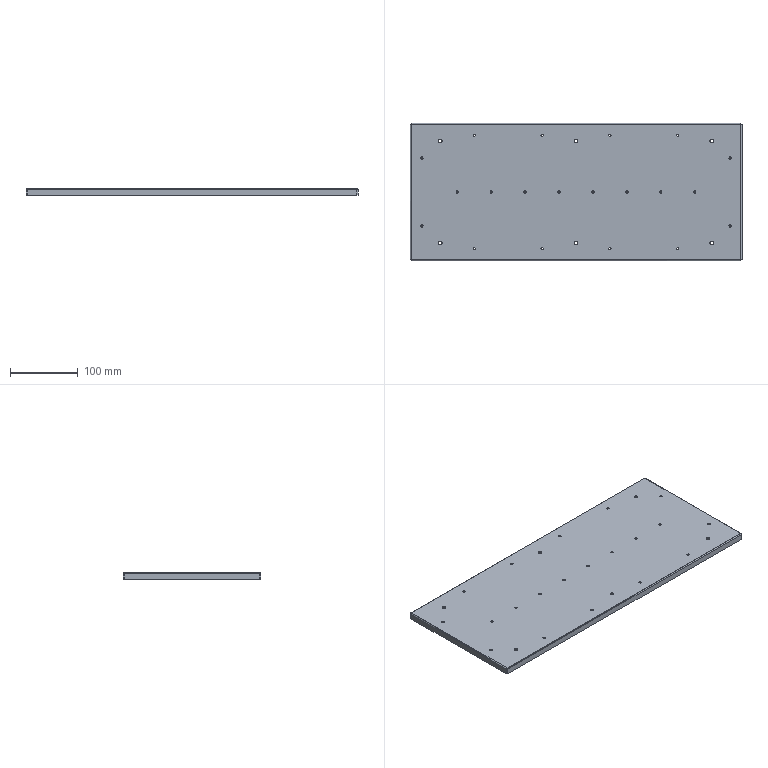Part | STEP file | 1 solid | 90 faces | box 489 x 202 x 10 mm | volume 164472 mm3 | cylinder 60 | plane 22 | spline 8 | commonest cylinder face diameters 3.3 x40 5.5 x12 0.02 x4 3.02 x4